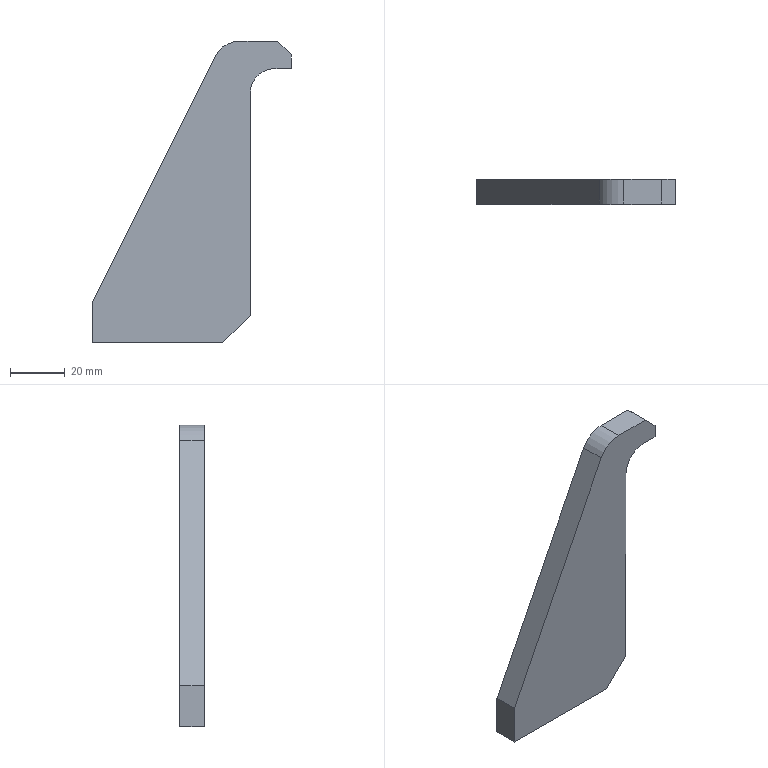Part | SolidWorks | features FlatPattern 1, SMBaseFlange 1, SheetMetal 1 | 1 solid | 13 faces | box 72.5 x 9 x 110 mm | volume 37505 mm3 | plane 11 | cylinder 2 | commonest cylinder face diameters 18 x1 20 x1
STEP:
#1=CARTESIAN_POINT('',(0.,0.,0.));
#2=VERTEX_POINT('',#1);
#3=CARTESIAN_POINT('',(0.,0.,15.));
#4=VERTEX_POINT('',#3);
#5=CARTESIAN_POINT('',(0.,0.,15.));
#6=DIRECTION('',(0.,0.,1.));
#7=VECTOR('',#6,1000.);
#8=LINE('',#5,#7);
#9=EDGE_CURVE('',#2,#4,#8,.T.);
#10=ORIENTED_EDGE('',*,*,#9,.F.);
#11=CARTESIAN_POINT('',(0.,-9.,0.));
#12=VERTEX_POINT('',#11);
#13=CARTESIAN_POINT('',(0.,-9.,0.));
#14=DIRECTION('',(0.,1.,0.));
#15=VECTOR('',#14,1000.);
#16=LINE('',#13,#15);
#17=EDGE_CURVE('',#12,#2,#16,.T.);
#18=ORIENTED_EDGE('',*,*,#17,.F.);
#19=CARTESIAN_POINT('',(0.,-9.,15.));
#20=VERTEX_POINT('',#19);
#21=CARTESIAN_POINT('',(0.,-9.,15.));
#22=DIRECTION('',(0.,0.,1.));
#23=VECTOR('',#22,1000.);
#24=LINE('',#21,#23);
#25=EDGE_CURVE('',#12,#20,#24,.T.);
#26=ORIENTED_EDGE('',*,*,#25,.T.);
#27=CARTESIAN_POINT('',(0.,-9.,15.));
#28=DIRECTION('',(0.,1.,0.));
#29=VECTOR('',#28,1000.);
#30=LINE('',#27,#29);
#31=EDGE_CURVE('',#20,#4,#30,.T.);
#32=ORIENTED_EDGE('',*,*,#31,.T.);
#33=EDGE_LOOP('',(#10,#18,#26,#32));
#34=FACE_OUTER_BOUND('',#33,.T.);
#35=CARTESIAN_POINT('',(0.,-9.,15.));
#36=DIRECTION('',(-1.,0.,0.));
#37=DIRECTION('',(0.,0.,1.));
#38=AXIS2_PLACEMENT_3D('',#35,#36,#37);
#39=PLANE('',#38);
#40=ADVANCED_FACE('',(#34),#39,.T.);
#41=CARTESIAN_POINT('',(47.5,0.,0.));
#42=VERTEX_POINT('',#41);
#43=CARTESIAN_POINT('',(0.,0.,0.));
#44=DIRECTION('',(-1.,0.,0.));
#45=VECTOR('',#44,1000.);
#46=LINE('',#43,#45);
#47=EDGE_CURVE('',#42,#2,#46,.T.);
#48=ORIENTED_EDGE('',*,*,#47,.F.);
#49=CARTESIAN_POINT('',(47.5,-9.,0.));
#50=VERTEX_POINT('',#49);
#51=CARTESIAN_POINT('',(47.5,-9.,0.));
#52=DIRECTION('',(0.,1.,0.));
#53=VECTOR('',#52,1000.);
#54=LINE('',#51,#53);
#55=EDGE_CURVE('',#50,#42,#54,.T.);
#56=ORIENTED_EDGE('',*,*,#55,.F.);
#57=CARTESIAN_POINT('',(0.,-9.,0.));
#58=DIRECTION('',(-1.,0.,0.));
#59=VECTOR('',#58,1000.);
#60=LINE('',#57,#59);
#61=EDGE_CURVE('',#50,#12,#60,.T.);
#62=ORIENTED_EDGE('',*,*,#61,.T.);
#63=ORIENTED_EDGE('',*,*,#17,.T.);
#64=EDGE_LOOP('',(#48,#56,#62,#63));
#65=FACE_OUTER_BOUND('',#64,.T.);
#66=CARTESIAN_POINT('',(0.,-9.,0.));
#67=DIRECTION('',(0.,0.,-1.));
#68=DIRECTION('',(-1.,0.,0.));
#69=AXIS2_PLACEMENT_3D('',#66,#67,#68);
#70=PLANE('',#69);
#71=ADVANCED_FACE('',(#65),#70,.T.);
#72=CARTESIAN_POINT('',(57.5,0.,10.));
#73=VERTEX_POINT('',#72);
#74=CARTESIAN_POINT('',(47.5,0.,0.));
#75=DIRECTION('',(-0.7071,0.,-0.7071));
#76=VECTOR('',#75,1000.);
#77=LINE('',#74,#76);
#78=EDGE_CURVE('',#73,#42,#77,.T.);
#79=ORIENTED_EDGE('',*,*,#78,.F.);
#80=CARTESIAN_POINT('',(57.5,-9.,10.));
#81=VERTEX_POINT('',#80);
#82=CARTESIAN_POINT('',(57.5,-9.,10.));
#83=DIRECTION('',(0.,1.,0.));
#84=VECTOR('',#83,1000.);
#85=LINE('',#82,#84);
#86=EDGE_CURVE('',#81,#73,#85,.T.);
#87=ORIENTED_EDGE('',*,*,#86,.F.);
#88=CARTESIAN_POINT('',(47.5,-9.,0.));
#89=DIRECTION('',(-0.7071,0.,-0.7071));
#90=VECTOR('',#89,1000.);
#91=LINE('',#88,#90);
#92=EDGE_CURVE('',#81,#50,#91,.T.);
#93=ORIENTED_EDGE('',*,*,#92,.T.);
#94=ORIENTED_EDGE('',*,*,#55,.T.);
#95=EDGE_LOOP('',(#79,#87,#93,#94));
#96=FACE_OUTER_BOUND('',#95,.T.);
#97=CARTESIAN_POINT('',(47.5,-9.,0.));
#98=DIRECTION('',(0.7071,0.,-0.7071));
#99=DIRECTION('',(-0.7071,0.,-0.7071));
#100=AXIS2_PLACEMENT_3D('',#97,#98,#99);
#101=PLANE('',#100);
#102=ADVANCED_FACE('',(#96),#101,.T.);
#103=CARTESIAN_POINT('',(57.5,0.,91.));
#104=VERTEX_POINT('',#103);
#105=CARTESIAN_POINT('',(57.5,0.,10.));
#106=DIRECTION('',(0.,0.,-1.));
#107=VECTOR('',#106,1000.);
#108=LINE('',#105,#107);
#109=EDGE_CURVE('',#104,#73,#108,.T.);
#110=ORIENTED_EDGE('',*,*,#109,.F.);
#111=CARTESIAN_POINT('',(57.5,-9.,91.));
#112=VERTEX_POINT('',#111);
#113=CARTESIAN_POINT('',(57.5,-9.,91.));
#114=DIRECTION('',(0.,1.,0.));
#115=VECTOR('',#114,1000.);
#116=LINE('',#113,#115);
#117=EDGE_CURVE('',#112,#104,#116,.T.);
#118=ORIENTED_EDGE('',*,*,#117,.F.);
#119=CARTESIAN_POINT('',(57.5,-9.,10.));
#120=DIRECTION('',(0.,0.,-1.));
#121=VECTOR('',#120,1000.);
#122=LINE('',#119,#121);
#123=EDGE_CURVE('',#112,#81,#122,.T.);
#124=ORIENTED_EDGE('',*,*,#123,.T.);
#125=ORIENTED_EDGE('',*,*,#86,.T.);
#126=EDGE_LOOP('',(#110,#118,#124,#125));
#127=FACE_OUTER_BOUND('',#126,.T.);
#128=CARTESIAN_POINT('',(57.5,-9.,10.));
#129=DIRECTION('',(1.,0.,0.));
#130=DIRECTION('',(0.,0.,-1.));
#131=AXIS2_PLACEMENT_3D('',#128,#129,#130);
#132=PLANE('',#131);
#133=ADVANCED_FACE('',(#127),#132,.T.);
#134=CARTESIAN_POINT('',(66.5,0.,100.));
#135=VERTEX_POINT('',#134);
#136=CARTESIAN_POINT('',(66.5,0.,91.));
#137=DIRECTION('',(0.,-1.,0.));
#138=DIRECTION('',(0.,0.,-1.));
#139=AXIS2_PLACEMENT_3D('',#136,#137,#138);
#140=CIRCLE('',#139,9.);
#141=EDGE_CURVE('',#135,#104,#140,.T.);
#142=ORIENTED_EDGE('',*,*,#141,.F.);
#143=CARTESIAN_POINT('',(66.5,-9.,100.));
#144=VERTEX_POINT('',#143);
#145=CARTESIAN_POINT('',(66.5,-9.,100.));
#146=DIRECTION('',(0.,1.,0.));
#147=VECTOR('',#146,1000.);
#148=LINE('',#145,#147);
#149=EDGE_CURVE('',#144,#135,#148,.T.);
#150=ORIENTED_EDGE('',*,*,#149,.F.);
#151=CARTESIAN_POINT('',(66.5,-9.,91.));
#152=DIRECTION('',(0.,-1.,0.));
#153=DIRECTION('',(0.,0.,-1.));
#154=AXIS2_PLACEMENT_3D('',#151,#152,#153);
#155=CIRCLE('',#154,9.);
#156=EDGE_CURVE('',#144,#112,#155,.T.);
#157=ORIENTED_EDGE('',*,*,#156,.T.);
#158=ORIENTED_EDGE('',*,*,#117,.T.);
#159=EDGE_LOOP('',(#142,#150,#157,#158));
#160=FACE_OUTER_BOUND('',#159,.T.);
#161=CARTESIAN_POINT('',(66.5,-9.,91.));
#162=DIRECTION('',(0.,1.,0.));
#163=DIRECTION('',(0.,0.,1.));
#164=AXIS2_PLACEMENT_3D('',#161,#162,#163);
#165=CYLINDRICAL_SURFACE('',#164,9.);
#166=ADVANCED_FACE('',(#160),#165,.F.);
#167=CARTESIAN_POINT('',(72.5,0.,100.));
#168=VERTEX_POINT('',#167);
#169=CARTESIAN_POINT('',(66.5,0.,100.));
#170=DIRECTION('',(-1.,0.,0.));
#171=VECTOR('',#170,1000.);
#172=LINE('',#169,#171);
#173=EDGE_CURVE('',#168,#135,#172,.T.);
#174=ORIENTED_EDGE('',*,*,#173,.F.);
#175=CARTESIAN_POINT('',(72.5,-9.,100.));
#176=VERTEX_POINT('',#175);
#177=CARTESIAN_POINT('',(72.5,-9.,100.));
#178=DIRECTION('',(0.,1.,0.));
#179=VECTOR('',#178,1000.);
#180=LINE('',#177,#179);
#181=EDGE_CURVE('',#176,#168,#180,.T.);
#182=ORIENTED_EDGE('',*,*,#181,.F.);
#183=CARTESIAN_POINT('',(66.5,-9.,100.));
#184=DIRECTION('',(-1.,0.,0.));
#185=VECTOR('',#184,1000.);
#186=LINE('',#183,#185);
#187=EDGE_CURVE('',#176,#144,#186,.T.);
#188=ORIENTED_EDGE('',*,*,#187,.T.);
#189=ORIENTED_EDGE('',*,*,#149,.T.);
#190=EDGE_LOOP('',(#174,#182,#188,#189));
#191=FACE_OUTER_BOUND('',#190,.T.);
#192=CARTESIAN_POINT('',(66.5,-9.,100.));
#193=DIRECTION('',(0.,0.,-1.));
#194=DIRECTION('',(-1.,0.,0.));
#195=AXIS2_PLACEMENT_3D('',#192,#193,#194);
#196=PLANE('',#195);
#197=ADVANCED_FACE('',(#191),#196,.T.);
#198=CARTESIAN_POINT('',(72.5,0.,105.));
#199=VERTEX_POINT('',#198);
#200=CARTESIAN_POINT('',(72.5,0.,100.));
#201=DIRECTION('',(0.,0.,-1.));
#202=VECTOR('',#201,1000.);
#203=LINE('',#200,#202);
#204=EDGE_CURVE('',#199,#168,#203,.T.);
#205=ORIENTED_EDGE('',*,*,#204,.F.);
#206=CARTESIAN_POINT('',(72.5,-9.,105.));
#207=VERTEX_POINT('',#206);
#208=CARTESIAN_POINT('',(72.5,-9.,105.));
#209=DIRECTION('',(0.,1.,0.));
#210=VECTOR('',#209,1000.);
#211=LINE('',#208,#210);
#212=EDGE_CURVE('',#207,#199,#211,.T.);
#213=ORIENTED_EDGE('',*,*,#212,.F.);
#214=CARTESIAN_POINT('',(72.5,-9.,100.));
#215=DIRECTION('',(0.,0.,-1.));
#216=VECTOR('',#215,1000.);
#217=LINE('',#214,#216);
#218=EDGE_CURVE('',#207,#176,#217,.T.);
#219=ORIENTED_EDGE('',*,*,#218,.T.);
#220=ORIENTED_EDGE('',*,*,#181,.T.);
#221=EDGE_LOOP('',(#205,#213,#219,#220));
#222=FACE_OUTER_BOUND('',#221,.T.);
#223=CARTESIAN_POINT('',(72.5,-9.,100.));
#224=DIRECTION('',(1.,0.,0.));
#225=DIRECTION('',(0.,0.,-1.));
#226=AXIS2_PLACEMENT_3D('',#223,#224,#225);
#227=PLANE('',#226);
#228=ADVANCED_FACE('',(#222),#227,.T.);
#229=CARTESIAN_POINT('',(67.5,0.,110.));
#230=VERTEX_POINT('',#229);
#231=CARTESIAN_POINT('',(72.5,0.,105.));
#232=DIRECTION('',(0.7071,0.,-0.7071));
#233=VECTOR('',#232,1000.);
#234=LINE('',#231,#233);
#235=EDGE_CURVE('',#230,#199,#234,.T.);
#236=ORIENTED_EDGE('',*,*,#235,.F.);
#237=CARTESIAN_POINT('',(67.5,-9.,110.));
#238=VERTEX_POINT('',#237);
#239=CARTESIAN_POINT('',(67.5,-9.,110.));
#240=DIRECTION('',(0.,1.,0.));
#241=VECTOR('',#240,1000.);
#242=LINE('',#239,#241);
#243=EDGE_CURVE('',#238,#230,#242,.T.);
#244=ORIENTED_EDGE('',*,*,#243,.F.);
#245=CARTESIAN_POINT('',(72.5,-9.,105.));
#246=DIRECTION('',(0.7071,0.,-0.7071));
#247=VECTOR('',#246,1000.);
#248=LINE('',#245,#247);
#249=EDGE_CURVE('',#238,#207,#248,.T.);
#250=ORIENTED_EDGE('',*,*,#249,.T.);
#251=ORIENTED_EDGE('',*,*,#212,.T.);
#252=EDGE_LOOP('',(#236,#244,#250,#251));
#253=FACE_OUTER_BOUND('',#252,.T.);
#254=CARTESIAN_POINT('',(72.5,-9.,105.));
#255=DIRECTION('',(0.7071,0.,0.7071));
#256=DIRECTION('',(0.7071,0.,-0.7071));
#257=AXIS2_PLACEMENT_3D('',#254,#255,#256);
#258=PLANE('',#257);
#259=ADVANCED_FACE('',(#253),#258,.T.);
#260=CARTESIAN_POINT('',(53.68,0.,110.));
#261=VERTEX_POINT('',#260);
#262=CARTESIAN_POINT('',(67.5,0.,110.));
#263=DIRECTION('',(1.,0.,0.));
#264=VECTOR('',#263,1000.);
#265=LINE('',#262,#264);
#266=EDGE_CURVE('',#261,#230,#265,.T.);
#267=ORIENTED_EDGE('',*,*,#266,.F.);
#268=CARTESIAN_POINT('',(53.68,-9.,110.));
#269=VERTEX_POINT('',#268);
#270=CARTESIAN_POINT('',(53.68,-9.,110.));
#271=DIRECTION('',(0.,1.,0.));
#272=VECTOR('',#271,1000.);
#273=LINE('',#270,#272);
#274=EDGE_CURVE('',#269,#261,#273,.T.);
#275=ORIENTED_EDGE('',*,*,#274,.F.);
#276=CARTESIAN_POINT('',(67.5,-9.,110.));
#277=DIRECTION('',(1.,0.,0.));
#278=VECTOR('',#277,1000.);
#279=LINE('',#276,#278);
#280=EDGE_CURVE('',#269,#238,#279,.T.);
#281=ORIENTED_EDGE('',*,*,#280,.T.);
#282=ORIENTED_EDGE('',*,*,#243,.T.);
#283=EDGE_LOOP('',(#267,#275,#281,#282));
#284=FACE_OUTER_BOUND('',#283,.T.);
#285=CARTESIAN_POINT('',(67.5,-9.,110.));
#286=DIRECTION('',(0.,0.,1.));
#287=DIRECTION('',(1.,0.,0.));
#288=AXIS2_PLACEMENT_3D('',#285,#286,#287);
#289=PLANE('',#288);
#290=ADVANCED_FACE('',(#284),#289,.T.);
#291=CARTESIAN_POINT('',(44.736,0.,104.472));
#292=VERTEX_POINT('',#291);
#293=CARTESIAN_POINT('',(53.68,0.,100.));
#294=DIRECTION('',(0.,1.,0.));
#295=DIRECTION('',(0.,0.,-1.));
#296=AXIS2_PLACEMENT_3D('',#293,#294,#295);
#297=CIRCLE('',#296,10.);
#298=EDGE_CURVE('',#292,#261,#297,.T.);
#299=ORIENTED_EDGE('',*,*,#298,.F.);
#300=CARTESIAN_POINT('',(44.736,-9.,104.472));
#301=VERTEX_POINT('',#300);
#302=CARTESIAN_POINT('',(44.736,-9.,104.472));
#303=DIRECTION('',(0.,1.,0.));
#304=VECTOR('',#303,1000.);
#305=LINE('',#302,#304);
#306=EDGE_CURVE('',#301,#292,#305,.T.);
#307=ORIENTED_EDGE('',*,*,#306,.F.);
#308=CARTESIAN_POINT('',(53.68,-9.,100.));
#309=DIRECTION('',(0.,1.,0.));
#310=DIRECTION('',(0.,0.,-1.));
#311=AXIS2_PLACEMENT_3D('',#308,#309,#310);
#312=CIRCLE('',#311,10.);
#313=EDGE_CURVE('',#301,#269,#312,.T.);
#314=ORIENTED_EDGE('',*,*,#313,.T.);
#315=ORIENTED_EDGE('',*,*,#274,.T.);
#316=EDGE_LOOP('',(#299,#307,#314,#315));
#317=FACE_OUTER_BOUND('',#316,.T.);
#318=CARTESIAN_POINT('',(53.68,-9.,100.));
#319=DIRECTION('',(0.,1.,0.));
#320=DIRECTION('',(0.,0.,1.));
#321=AXIS2_PLACEMENT_3D('',#318,#319,#320);
#322=CYLINDRICAL_SURFACE('',#321,10.);
#323=ADVANCED_FACE('',(#317),#322,.T.);
#324=CARTESIAN_POINT('',(44.736,0.,104.472));
#325=DIRECTION('',(0.4472,0.,0.8944));
#326=VECTOR('',#325,1000.);
#327=LINE('',#324,#326);
#328=EDGE_CURVE('',#4,#292,#327,.T.);
#329=ORIENTED_EDGE('',*,*,#328,.F.);
#330=ORIENTED_EDGE('',*,*,#31,.F.);
#331=CARTESIAN_POINT('',(44.736,-9.,104.472));
#332=DIRECTION('',(0.4472,0.,0.8944));
#333=VECTOR('',#332,1000.);
#334=LINE('',#331,#333);
#335=EDGE_CURVE('',#20,#301,#334,.T.);
#336=ORIENTED_EDGE('',*,*,#335,.T.);
#337=ORIENTED_EDGE('',*,*,#306,.T.);
#338=EDGE_LOOP('',(#329,#330,#336,#337));
#339=FACE_OUTER_BOUND('',#338,.T.);
#340=CARTESIAN_POINT('',(44.736,-9.,104.472));
#341=DIRECTION('',(-0.8944,0.,0.4472));
#342=DIRECTION('',(0.4472,0.,0.8944));
#343=AXIS2_PLACEMENT_3D('',#340,#341,#342);
#344=PLANE('',#343);
#345=ADVANCED_FACE('',(#339),#344,.T.);
#346=ORIENTED_EDGE('',*,*,#25,.F.);
#347=ORIENTED_EDGE('',*,*,#61,.F.);
#348=ORIENTED_EDGE('',*,*,#92,.F.);
#349=ORIENTED_EDGE('',*,*,#123,.F.);
#350=ORIENTED_EDGE('',*,*,#156,.F.);
#351=ORIENTED_EDGE('',*,*,#187,.F.);
#352=ORIENTED_EDGE('',*,*,#218,.F.);
#353=ORIENTED_EDGE('',*,*,#249,.F.);
#354=ORIENTED_EDGE('',*,*,#280,.F.);
#355=ORIENTED_EDGE('',*,*,#313,.F.);
#356=ORIENTED_EDGE('',*,*,#335,.F.);
#357=EDGE_LOOP('',(#346,#347,#348,#349,#350,#351,#352,#353,#354,#355,#356));
#358=FACE_OUTER_BOUND('',#357,.T.);
#359=CARTESIAN_POINT('',(66.5,-9.,91.));
#360=DIRECTION('',(0.,-1.,0.));
#361=DIRECTION('',(0.,0.,-1.));
#362=AXIS2_PLACEMENT_3D('',#359,#360,#361);
#363=PLANE('',#362);
#364=ADVANCED_FACE('',(#358),#363,.T.);
#365=ORIENTED_EDGE('',*,*,#9,.T.);
#366=ORIENTED_EDGE('',*,*,#328,.T.);
#367=ORIENTED_EDGE('',*,*,#298,.T.);
#368=ORIENTED_EDGE('',*,*,#266,.T.);
#369=ORIENTED_EDGE('',*,*,#235,.T.);
#370=ORIENTED_EDGE('',*,*,#204,.T.);
#371=ORIENTED_EDGE('',*,*,#173,.T.);
#372=ORIENTED_EDGE('',*,*,#141,.T.);
#373=ORIENTED_EDGE('',*,*,#109,.T.);
#374=ORIENTED_EDGE('',*,*,#78,.T.);
#375=ORIENTED_EDGE('',*,*,#47,.T.);
#376=EDGE_LOOP('',(#365,#366,#367,#368,#369,#370,#371,#372,#373,#374,#375));
#377=FACE_OUTER_BOUND('',#376,.T.);
#378=CARTESIAN_POINT('',(66.5,0.,91.));
#379=DIRECTION('',(0.,-1.,0.));
#380=DIRECTION('',(0.,0.,-1.));
#381=AXIS2_PLACEMENT_3D('',#378,#379,#380);
#382=PLANE('',#381);
#383=ADVANCED_FACE('',(#377),#382,.F.);
#384=CLOSED_SHELL('',(#40,#71,#102,#133,#166,#197,#228,#259,#290,#323,#345,#364,#383));
#385=MANIFOLD_SOLID_BREP('',#384);
#386=CARTESIAN_POINT('',(0.,0.,0.));
#387=DIRECTION('',(0.,0.,1.));
#388=DIRECTION('',(1.,0.,0.));
#389=AXIS2_PLACEMENT_3D('',#386,#387,#388);
#390=(LENGTH_UNIT()NAMED_UNIT(*)SI_UNIT(.MILLI.,.METRE.));
#391=UNCERTAINTY_MEASURE_WITH_UNIT(LENGTH_MEASURE(0.00001),#390,'','');
#392=(NAMED_UNIT(*)PLANE_ANGLE_UNIT()SI_UNIT($,.RADIAN.));
#393=(NAMED_UNIT(*)SI_UNIT($,.STERADIAN.)SOLID_ANGLE_UNIT());
#394=(GEOMETRIC_REPRESENTATION_CONTEXT(3)GLOBAL_UNCERTAINTY_ASSIGNED_CONTEXT((#391))GLOBAL_UNIT_ASSIGNED_CONTEXT((#390,#392,#393))REPRESENTATION_CONTEXT('',''));
#395=ADVANCED_BREP_SHAPE_REPRESENTATION('',(#385,#389),#394);